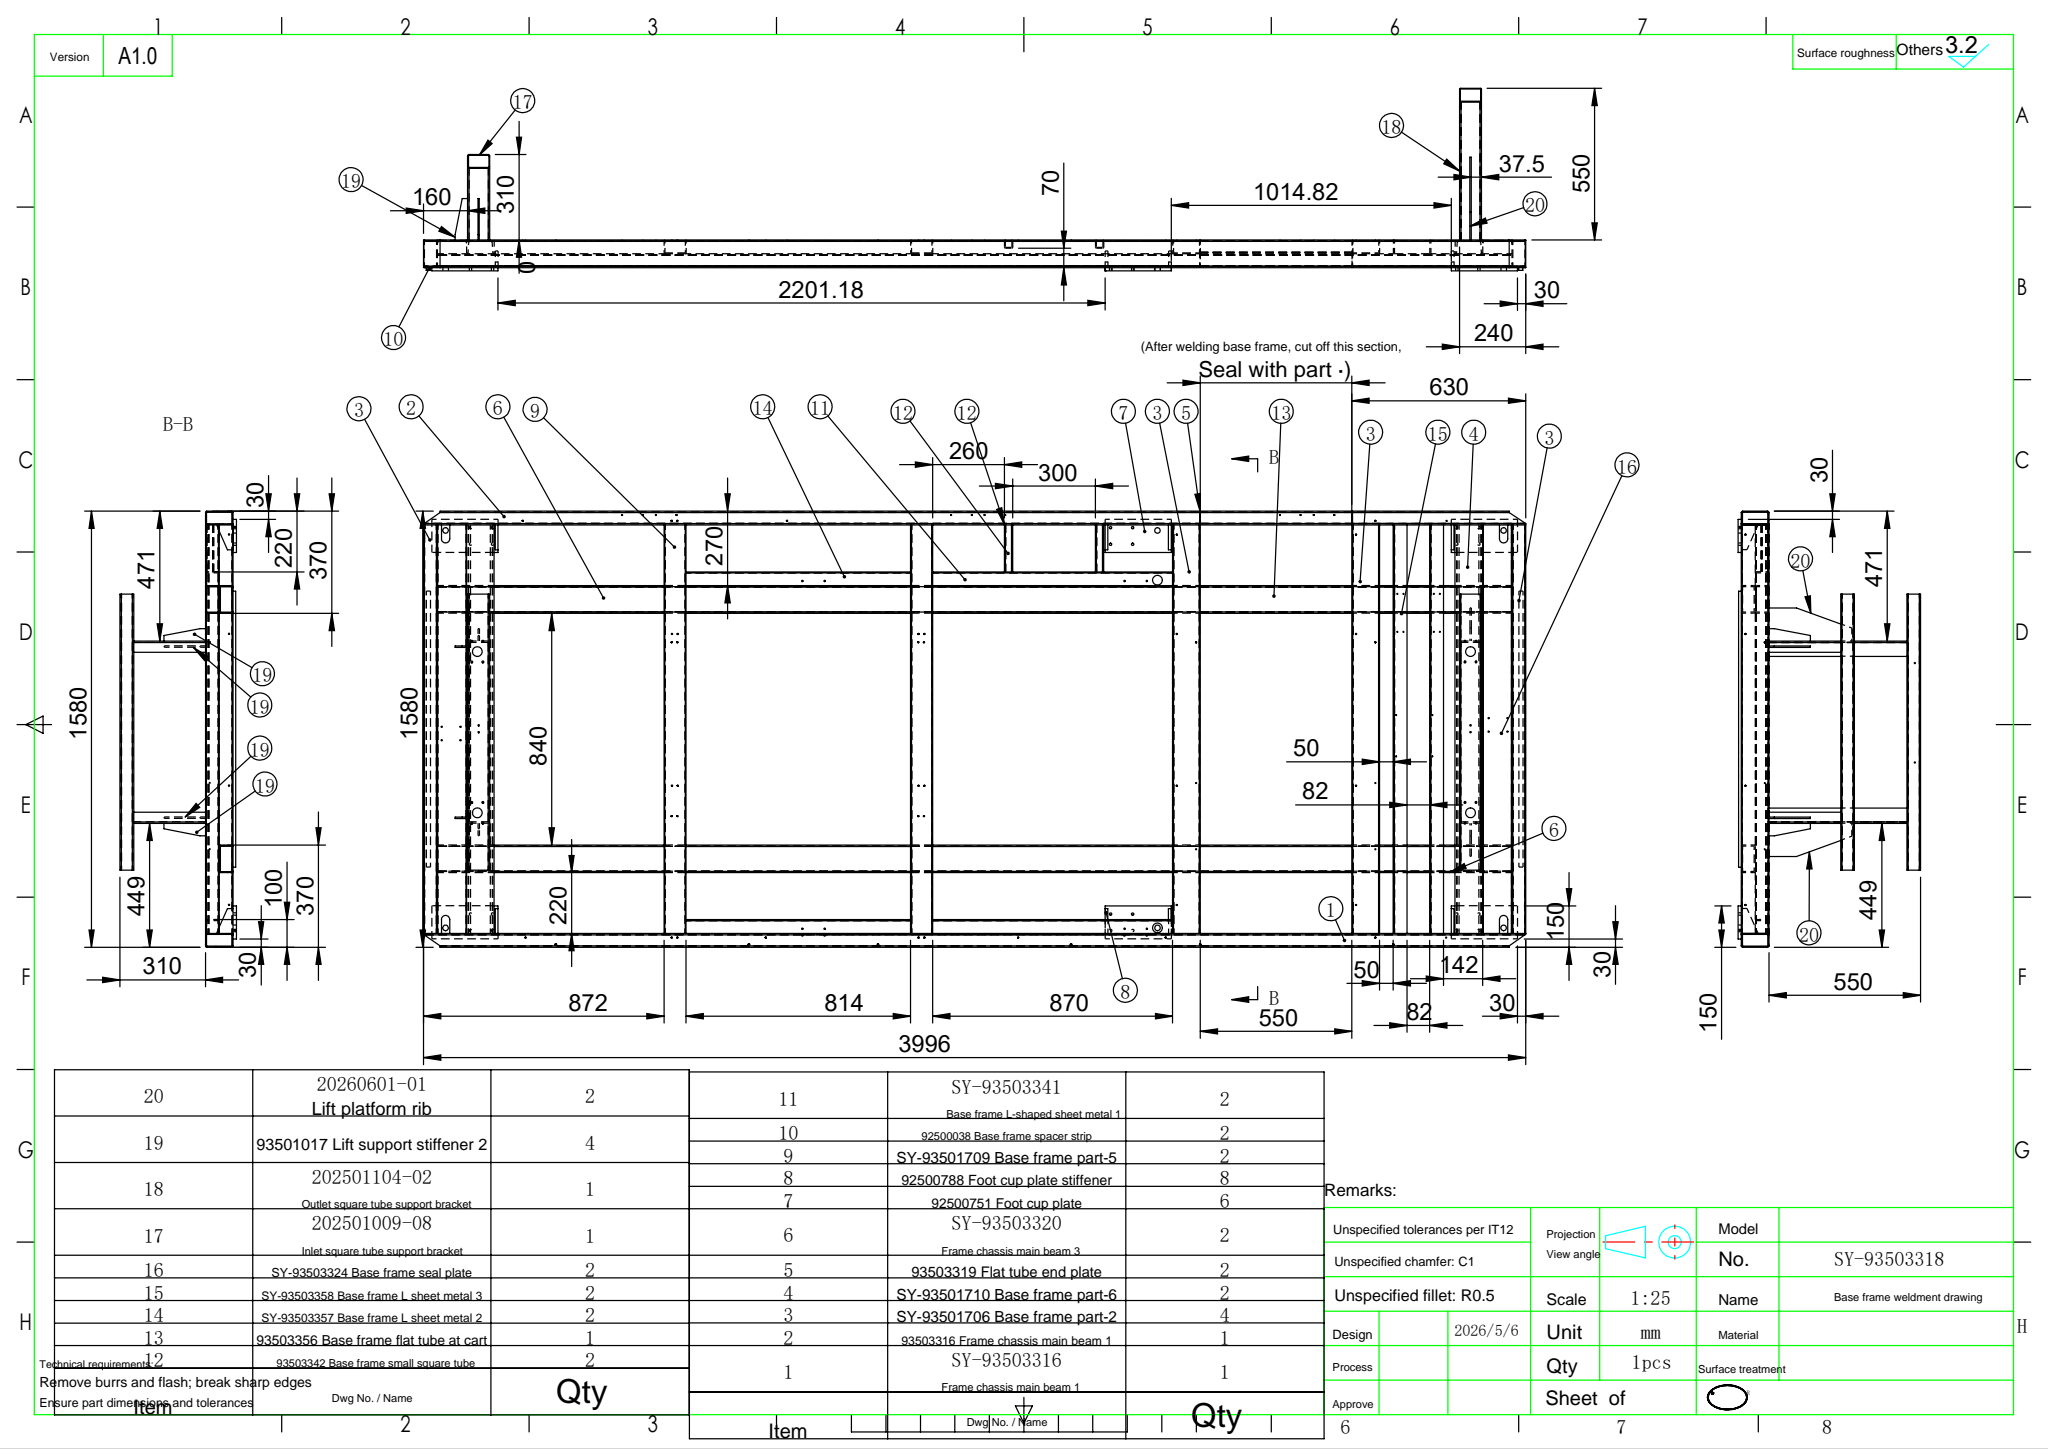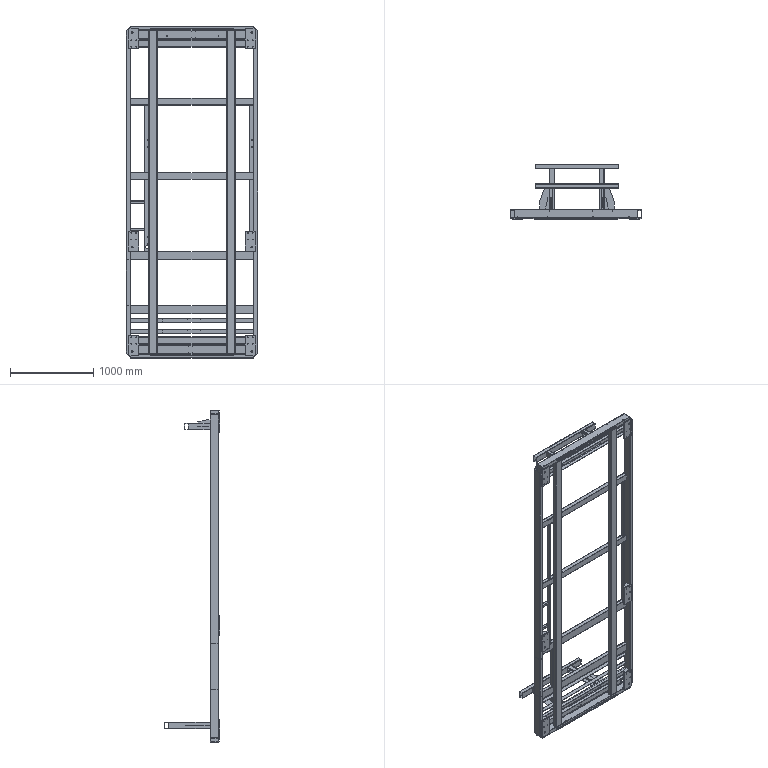Part | SolidWorks | 54 solids | 1175 faces | box 1580 x 662 x 3996 mm | volume 37221159 mm3 | cylinder 520 | plane 519 | cone 136 | commonest cylinder face diameters 3.3 x136 8.5 x48 10 x48 5 x44 0.4 x38 2 x32